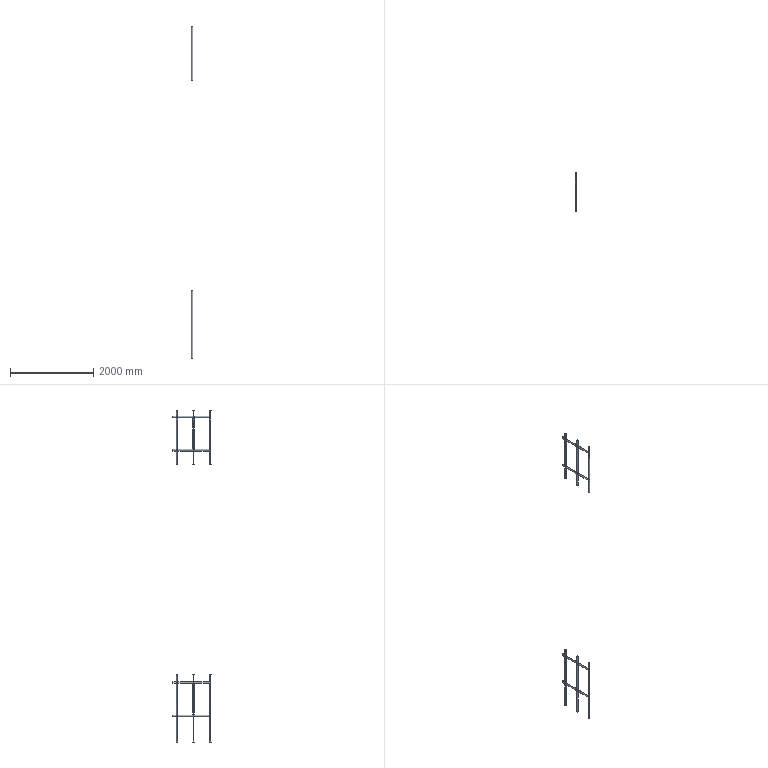Part | NX | features BREP 2 | 2 solids | 96 faces | box 40 x 920 x 7998 mm | volume 15170680 mm3 | cylinder 56 | plane 40 | commonest cylinder face diameters 40 x56